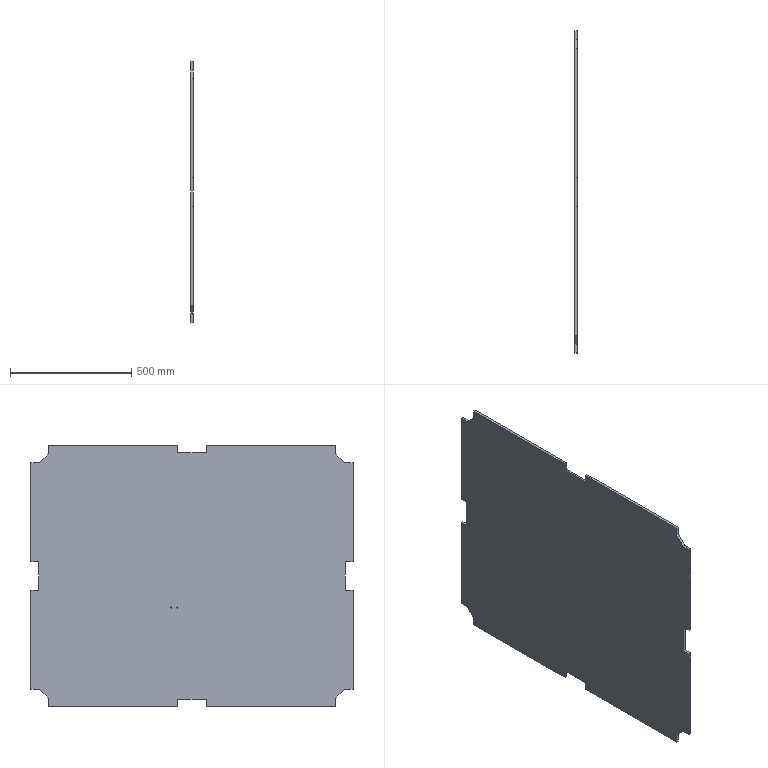Part | STEP file | 01-10 Base plate 2 | 1 solid | 38 faces | box 10 x 1330 x 1080 mm | volume 14031243 mm3 | plane 34 | cylinder 4 | commonest cylinder face diameters 4.2 x4